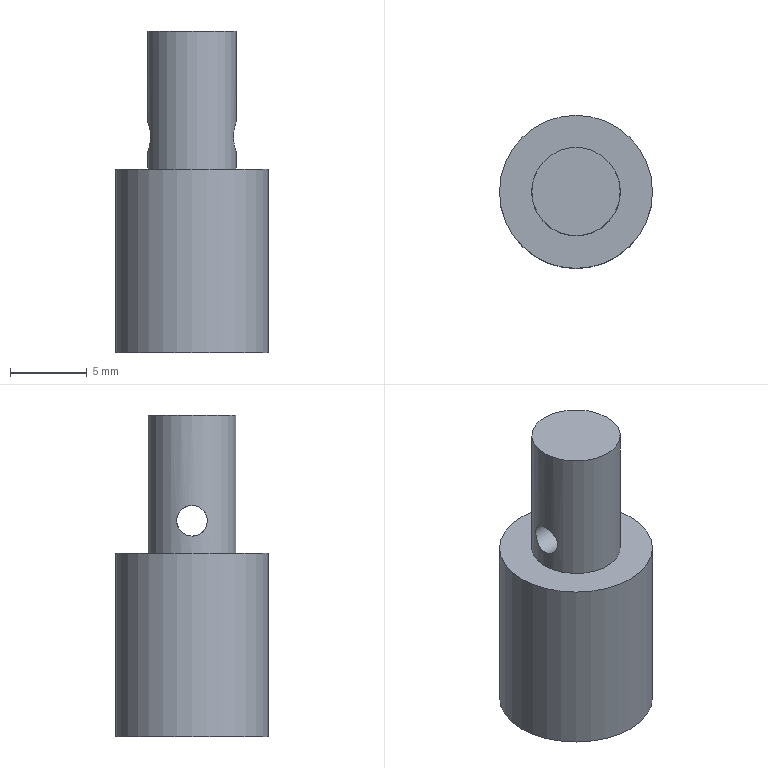Part | STEP file | Ground post | 1 solid | 6 faces | box 10 x 10 x 21 mm | volume 1161 mm3 | cylinder 3 | plane 3 | commonest cylinder face diameters 2 x1 5.78 x1 10 x1
STEP:
#1=CARTESIAN_POINT('',(0.,0.,0.));
#2=DIRECTION('',(0.,0.,1.));
#3=DIRECTION('',(1.,0.,0.));
#4=AXIS2_PLACEMENT_3D('',#1,#2,#3);
#5=CARTESIAN_POINT('',(2.89,0.,11.));
#6=VERTEX_POINT('',#5);
#7=CARTESIAN_POINT('',(0.,0.,11.));
#8=DIRECTION('',(0.,0.,1.));
#9=DIRECTION('',(1.,0.,0.));
#10=AXIS2_PLACEMENT_3D('',#7,#8,#9);
#11=CIRCLE('',#10,2.89);
#12=CARTESIAN_POINT('',(0.,0.,11.));
#13=DIRECTION('',(0.,0.,-1.));
#14=DIRECTION('',(-1.,0.,0.));
#15=AXIS2_PLACEMENT_3D('',#12,#13,#14);
#16=CYLINDRICAL_SURFACE('',#15,2.89);
#17=CARTESIAN_POINT('',(9.425,0.));
#18=DIRECTION('',(-1.,0.));
#19=VECTOR('',#18,1.);
#20=LINE('',#17,#19);
#21=(GEOMETRIC_REPRESENTATION_CONTEXT(2)PARAMETRIC_REPRESENTATION_CONTEXT()REPRESENTATION_CONTEXT('',''));
#22=DEFINITIONAL_REPRESENTATION('',(#20),#21);
#23=PCURVE('',#16,#22);
#24=CARTESIAN_POINT('',(0.,0.,11.));
#25=DIRECTION('',(0.,0.,1.));
#26=DIRECTION('',(1.,0.,0.));
#27=AXIS2_PLACEMENT_3D('',#24,#25,#26);
#28=PLANE('',#27);
#29=CARTESIAN_POINT('',(0.,0.));
#30=DIRECTION('',(1.,0.));
#31=AXIS2_PLACEMENT_2D('',#29,#30);
#32=CIRCLE('',#31,2.89);
#33=(GEOMETRIC_REPRESENTATION_CONTEXT(2)PARAMETRIC_REPRESENTATION_CONTEXT()REPRESENTATION_CONTEXT('',''));
#34=DEFINITIONAL_REPRESENTATION('',(#32),#33);
#35=PCURVE('',#28,#34);
#36=SURFACE_CURVE('',#11,(#23,#35),.PCURVE_S1.);
#37=EDGE_CURVE('',#6,#6,#36,.T.);
#38=ORIENTED_EDGE('',*,*,#37,.F.);
#39=CARTESIAN_POINT('',(2.89,0.,5.108));
#40=VERTEX_POINT('',#39);
#41=CARTESIAN_POINT('',(2.89,0.,11.));
#42=CARTESIAN_POINT('',(2.89,0.,5.108));
#43=B_SPLINE_CURVE_WITH_KNOTS('',1,(#41,#42),.UNSPECIFIED.,.F.,.F.,(2,2),(0.,5.892),.PIECEWISE_BEZIER_KNOTS.);
#44=CARTESIAN_POINT('',(9.425,0.));
#45=DIRECTION('',(0.,1.));
#46=VECTOR('',#45,1.);
#47=LINE('',#44,#46);
#48=(GEOMETRIC_REPRESENTATION_CONTEXT(2)PARAMETRIC_REPRESENTATION_CONTEXT()REPRESENTATION_CONTEXT('',''));
#49=DEFINITIONAL_REPRESENTATION('',(#47),#48);
#50=PCURVE('',#16,#49);
#51=CARTESIAN_POINT('',(3.142,0.));
#52=DIRECTION('',(0.,1.));
#53=VECTOR('',#52,1.);
#54=LINE('',#51,#53);
#55=(GEOMETRIC_REPRESENTATION_CONTEXT(2)PARAMETRIC_REPRESENTATION_CONTEXT()REPRESENTATION_CONTEXT('',''));
#56=DEFINITIONAL_REPRESENTATION('',(#54),#55);
#57=PCURVE('',#16,#56);
#58=SEAM_CURVE('',#43,(#50,#57),.PCURVE_S1.);
#59=EDGE_CURVE('',#6,#40,#58,.T.);
#60=ORIENTED_EDGE('',*,*,#59,.T.);
#61=CARTESIAN_POINT('',(2.89,0.,3.108));
#62=VERTEX_POINT('',#61);
#63=CARTESIAN_POINT('',(2.89,0.,5.108));
#64=CARTESIAN_POINT('',(2.89,-0.1084,5.108));
#65=CARTESIAN_POINT('',(2.884,-0.2182,5.09));
#66=CARTESIAN_POINT('',(2.872,-0.3203,5.055));
#67=CARTESIAN_POINT('',(2.861,-0.4222,5.021));
#68=CARTESIAN_POINT('',(2.844,-0.5192,4.969));
#69=CARTESIAN_POINT('',(2.826,-0.6042,4.904));
#70=CARTESIAN_POINT('',(2.807,-0.6921,4.838));
#71=CARTESIAN_POINT('',(2.786,-0.7695,4.756));
#72=CARTESIAN_POINT('',(2.768,-0.8309,4.664));
#73=CARTESIAN_POINT('',(2.749,-0.8942,4.57));
#74=CARTESIAN_POINT('',(2.732,-0.9421,4.462));
#75=CARTESIAN_POINT('',(2.722,-0.97,4.351));
#76=CARTESIAN_POINT('',(2.713,-0.9969,4.243));
#77=CARTESIAN_POINT('',(2.709,-1.006,4.129));
#78=CARTESIAN_POINT('',(2.713,-0.996,4.019));
#79=CARTESIAN_POINT('',(2.716,-0.9866,3.913));
#80=CARTESIAN_POINT('',(2.726,-0.96,3.809));
#81=CARTESIAN_POINT('',(2.74,-0.9186,3.712));
#82=CARTESIAN_POINT('',(2.754,-0.8765,3.615));
#83=CARTESIAN_POINT('',(2.773,-0.8181,3.523));
#84=CARTESIAN_POINT('',(2.792,-0.7479,3.444));
#85=CARTESIAN_POINT('',(2.811,-0.6737,3.36));
#86=CARTESIAN_POINT('',(2.832,-0.5842,3.288));
#87=CARTESIAN_POINT('',(2.849,-0.4861,3.234));
#88=CARTESIAN_POINT('',(2.866,-0.3869,3.179));
#89=CARTESIAN_POINT('',(2.879,-0.2759,3.14));
#90=CARTESIAN_POINT('',(2.885,-0.1628,3.121));
#91=CARTESIAN_POINT('',(2.891,-0.05501,3.103));
#92=CARTESIAN_POINT('',(2.891,0.05773,3.103));
#93=CARTESIAN_POINT('',(2.885,0.1655,3.121));
#94=CARTESIAN_POINT('',(2.879,0.2699,3.139));
#95=CARTESIAN_POINT('',(2.867,0.3724,3.174));
#96=CARTESIAN_POINT('',(2.852,0.4652,3.222));
#97=CARTESIAN_POINT('',(2.837,0.5607,3.273));
#98=CARTESIAN_POINT('',(2.817,0.6485,3.339));
#99=CARTESIAN_POINT('',(2.798,0.7227,3.416));
#100=CARTESIAN_POINT('',(2.778,0.8004,3.498));
#101=CARTESIAN_POINT('',(2.758,0.8653,3.594));
#102=CARTESIAN_POINT('',(2.742,0.9118,3.697));
#103=CARTESIAN_POINT('',(2.727,0.9582,3.8));
#104=CARTESIAN_POINT('',(2.716,0.9876,3.914));
#105=CARTESIAN_POINT('',(2.713,0.9968,4.027));
#106=CARTESIAN_POINT('',(2.709,1.005,4.135));
#107=CARTESIAN_POINT('',(2.713,0.9963,4.245));
#108=CARTESIAN_POINT('',(2.722,0.9703,4.35));
#109=CARTESIAN_POINT('',(2.731,0.9448,4.452));
#110=CARTESIAN_POINT('',(2.746,0.9027,4.55));
#111=CARTESIAN_POINT('',(2.763,0.8474,4.639));
#112=CARTESIAN_POINT('',(2.781,0.7896,4.731));
#113=CARTESIAN_POINT('',(2.801,0.7157,4.814));
#114=CARTESIAN_POINT('',(2.82,0.6314,4.883));
#115=CARTESIAN_POINT('',(2.84,0.5434,4.955));
#116=CARTESIAN_POINT('',(2.858,0.4413,5.012));
#117=CARTESIAN_POINT('',(2.871,0.3333,5.05));
#118=CARTESIAN_POINT('',(2.883,0.2275,5.088));
#119=CARTESIAN_POINT('',(2.89,0.1129,5.108));
#120=CARTESIAN_POINT('',(2.89,0.,5.108));
#121=B_SPLINE_CURVE_WITH_KNOTS('',3,(#63,#64,#65,#66,#67,#68,#69,#70,#71,#72,#73,#74,#75,#76,#77,#78,#79,#80,#81,#82,#83,#84,#85,#86,#87,#88,#89,#90,#91,#92,#93,#94,#95,#96,#97,#98,#99,#100,#101,#102,#103,#104,#105,#106,#107,#108,#109,#110,#111,#112,#113,#114,#115,#116,#117,#118,#119,#120),.UNSPECIFIED.,.T.,.F.,(1,3,3,3,3,3,3,3,3,3,3,3,3,3,3,3,3,3,3,3,3,1),(-0.0538,0.,0.05159,0.1031,0.1563,0.2112,0.2642,0.3144,0.3655,0.4195,0.4742,0.5263,0.5767,0.6285,0.6829,0.7374,0.7887,0.8388,0.8913,0.9462,1.,1.052),.UNSPECIFIED.);
#122=CARTESIAN_POINT('',(9.425,5.892));
#123=CARTESIAN_POINT('',(9.433,5.892));
#124=CARTESIAN_POINT('',(9.45,5.894));
#125=CARTESIAN_POINT('',(9.474,5.902));
#126=CARTESIAN_POINT('',(9.499,5.915));
#127=CARTESIAN_POINT('',(9.523,5.933));
#128=CARTESIAN_POINT('',(9.547,5.955));
#129=CARTESIAN_POINT('',(9.57,5.983));
#130=CARTESIAN_POINT('',(9.592,6.015));
#131=CARTESIAN_POINT('',(9.614,6.051));
#132=CARTESIAN_POINT('',(9.634,6.092));
#133=CARTESIAN_POINT('',(9.654,6.136));
#134=CARTESIAN_POINT('',(9.672,6.185));
#135=CARTESIAN_POINT('',(9.69,6.237));
#136=CARTESIAN_POINT('',(9.706,6.292));
#137=CARTESIAN_POINT('',(9.72,6.35));
#138=CARTESIAN_POINT('',(9.733,6.411));
#139=CARTESIAN_POINT('',(9.745,6.475));
#140=CARTESIAN_POINT('',(9.755,6.541));
#141=CARTESIAN_POINT('',(9.763,6.609));
#142=CARTESIAN_POINT('',(9.77,6.678));
#143=CARTESIAN_POINT('',(9.775,6.748));
#144=CARTESIAN_POINT('',(9.777,6.82));
#145=CARTESIAN_POINT('',(9.778,6.892));
#146=CARTESIAN_POINT('',(9.777,6.964));
#147=CARTESIAN_POINT('',(9.775,7.035));
#148=CARTESIAN_POINT('',(9.77,7.106));
#149=CARTESIAN_POINT('',(9.763,7.176));
#150=CARTESIAN_POINT('',(9.755,7.244));
#151=CARTESIAN_POINT('',(9.745,7.309));
#152=CARTESIAN_POINT('',(9.733,7.373));
#153=CARTESIAN_POINT('',(9.72,7.434));
#154=CARTESIAN_POINT('',(9.705,7.493));
#155=CARTESIAN_POINT('',(9.689,7.548));
#156=CARTESIAN_POINT('',(9.672,7.6));
#157=CARTESIAN_POINT('',(9.654,7.648));
#158=CARTESIAN_POINT('',(9.634,7.693));
#159=CARTESIAN_POINT('',(9.614,7.733));
#160=CARTESIAN_POINT('',(9.592,7.77));
#161=CARTESIAN_POINT('',(9.57,7.802));
#162=CARTESIAN_POINT('',(9.547,7.829));
#163=CARTESIAN_POINT('',(9.523,7.852));
#164=CARTESIAN_POINT('',(9.499,7.87));
#165=CARTESIAN_POINT('',(9.475,7.883));
#166=CARTESIAN_POINT('',(9.45,7.89));
#167=CARTESIAN_POINT('',(9.425,7.893));
#168=CARTESIAN_POINT('',(9.4,7.891));
#169=CARTESIAN_POINT('',(9.375,7.883));
#170=CARTESIAN_POINT('',(9.351,7.87));
#171=CARTESIAN_POINT('',(9.327,7.852));
#172=CARTESIAN_POINT('',(9.303,7.829));
#173=CARTESIAN_POINT('',(9.28,7.802));
#174=CARTESIAN_POINT('',(9.258,7.77));
#175=CARTESIAN_POINT('',(9.236,7.734));
#176=CARTESIAN_POINT('',(9.215,7.693));
#177=CARTESIAN_POINT('',(9.196,7.648));
#178=CARTESIAN_POINT('',(9.177,7.6));
#179=CARTESIAN_POINT('',(9.16,7.548));
#180=CARTESIAN_POINT('',(9.144,7.493));
#181=CARTESIAN_POINT('',(9.129,7.434));
#182=CARTESIAN_POINT('',(9.116,7.373));
#183=CARTESIAN_POINT('',(9.105,7.31));
#184=CARTESIAN_POINT('',(9.095,7.244));
#185=CARTESIAN_POINT('',(9.086,7.176));
#186=CARTESIAN_POINT('',(9.08,7.107));
#187=CARTESIAN_POINT('',(9.075,7.036));
#188=CARTESIAN_POINT('',(9.072,6.965));
#189=CARTESIAN_POINT('',(9.071,6.893));
#190=CARTESIAN_POINT('',(9.072,6.821));
#191=CARTESIAN_POINT('',(9.075,6.749));
#192=CARTESIAN_POINT('',(9.08,6.678));
#193=CARTESIAN_POINT('',(9.086,6.609));
#194=CARTESIAN_POINT('',(9.095,6.541));
#195=CARTESIAN_POINT('',(9.105,6.475));
#196=CARTESIAN_POINT('',(9.116,6.411));
#197=CARTESIAN_POINT('',(9.129,6.35));
#198=CARTESIAN_POINT('',(9.144,6.292));
#199=CARTESIAN_POINT('',(9.16,6.237));
#200=CARTESIAN_POINT('',(9.177,6.185));
#201=CARTESIAN_POINT('',(9.196,6.136));
#202=CARTESIAN_POINT('',(9.215,6.092));
#203=CARTESIAN_POINT('',(9.236,6.051));
#204=CARTESIAN_POINT('',(9.258,6.015));
#205=CARTESIAN_POINT('',(9.28,5.983));
#206=CARTESIAN_POINT('',(9.303,5.955));
#207=CARTESIAN_POINT('',(9.326,5.933));
#208=CARTESIAN_POINT('',(9.351,5.915));
#209=CARTESIAN_POINT('',(9.375,5.902));
#210=CARTESIAN_POINT('',(9.4,5.894));
#211=CARTESIAN_POINT('',(9.417,5.892));
#212=CARTESIAN_POINT('',(9.425,5.892));
#213=B_SPLINE_CURVE_WITH_KNOTS('',3,(#122,#123,#124,#125,#126,#127,#128,#129,#130,#131,#132,#133,#134,#135,#136,#137,#138,#139,#140,#141,#142,#143,#144,#145,#146,#147,#148,#149,#150,#151,#152,#153,#154,#155,#156,#157,#158,#159,#160,#161,#162,#163,#164,#165,#166,#167,#168,#169,#170,#171,#172,#173,#174,#175,#176,#177,#178,#179,#180,#181,#182,#183,#184,#185,#186,#187,#188,#189,#190,#191,#192,#193,#194,#195,#196,#197,#198,#199,#200,#201,#202,#203,#204,#205,#206,#207,#208,#209,#210,#211,#212),.UNSPECIFIED.,.T.,.F.,(4,1,1,1,1,1,1,1,1,1,1,1,1,1,1,1,1,1,1,1,1,1,1,1,1,1,1,1,1,1,1,1,1,1,1,1,1,1,1,1,1,1,1,1,1,1,1,1,1,1,1,1,1,1,1,1,1,1,1,1,1,1,1,1,1,1,1,1,1,1,1,1,1,1,1,1,1,1,1,1,1,1,1,1,1,1,1,1,4),(0.,0.01136,0.02273,0.03409,0.04545,0.05682,0.06818,0.07955,0.09091,0.1023,0.1136,0.125,0.1364,0.1477,0.1591,0.1705,0.1818,0.1932,0.2045,0.2159,0.2273,0.2386,0.25,0.2614,0.2727,0.2841,0.2955,0.3068,0.3182,0.3295,0.3409,0.3523,0.3636,0.375,0.3864,0.3977,0.4091,0.4205,0.4318,0.4432,0.4545,0.4659,0.4773,0.4886,0.5,0.5114,0.5227,0.5341,0.5455,0.5568,0.5682,0.5795,0.5909,0.6023,0.6136,0.625,0.6364,0.6477,0.6591,0.6705,0.6818,0.6932,0.7045,0.7159,0.7273,0.7386,0.75,0.7614,0.7727,0.7841,0.7955,0.8068,0.8182,0.8295,0.8409,0.8523,0.8636,0.875,0.8864,0.8977,0.9091,0.9205,0.9318,0.9432,0.9545,0.9659,0.9773,0.9886,1.),.QUASI_UNIFORM_KNOTS.);
#214=(GEOMETRIC_REPRESENTATION_CONTEXT(2)PARAMETRIC_REPRESENTATION_CONTEXT()REPRESENTATION_CONTEXT('',''));
#215=DEFINITIONAL_REPRESENTATION('',(#213),#214);
#216=PCURVE('',#16,#215);
#217=CARTESIAN_POINT('',(10.,0.,4.108));
#218=DIRECTION('',(-1.,0.,0.));
#219=DIRECTION('',(0.,0.,1.));
#220=AXIS2_PLACEMENT_3D('',#217,#218,#219);
#221=CYLINDRICAL_SURFACE('',#220,1.);
#222=CARTESIAN_POINT('',(3.142,7.11));
#223=CARTESIAN_POINT('',(3.118,7.11));
#224=CARTESIAN_POINT('',(3.069,7.111));
#225=CARTESIAN_POINT('',(2.998,7.113));
#226=CARTESIAN_POINT('',(2.926,7.118));
#227=CARTESIAN_POINT('',(2.854,7.124));
#228=CARTESIAN_POINT('',(2.782,7.131));
#229=CARTESIAN_POINT('',(2.711,7.14));
#230=CARTESIAN_POINT('',(2.64,7.15));
#231=CARTESIAN_POINT('',(2.569,7.161));
#232=CARTESIAN_POINT('',(2.498,7.173));
#233=CARTESIAN_POINT('',(2.426,7.185));
#234=CARTESIAN_POINT('',(2.356,7.198));
#235=CARTESIAN_POINT('',(2.285,7.211));
#236=CARTESIAN_POINT('',(2.214,7.223));
#237=CARTESIAN_POINT('',(2.143,7.235));
#238=CARTESIAN_POINT('',(2.072,7.246));
#239=CARTESIAN_POINT('',(2.001,7.257));
#240=CARTESIAN_POINT('',(1.93,7.266));
#241=CARTESIAN_POINT('',(1.858,7.274));
#242=CARTESIAN_POINT('',(1.786,7.28));
#243=CARTESIAN_POINT('',(1.714,7.285));
#244=CARTESIAN_POINT('',(1.643,7.288));
#245=CARTESIAN_POINT('',(1.571,7.289));
#246=CARTESIAN_POINT('',(1.499,7.288));
#247=CARTESIAN_POINT('',(1.427,7.285));
#248=CARTESIAN_POINT('',(1.355,7.28));
#249=CARTESIAN_POINT('',(1.284,7.274));
#250=CARTESIAN_POINT('',(1.212,7.266));
#251=CARTESIAN_POINT('',(1.14,7.257));
#252=CARTESIAN_POINT('',(1.069,7.246));
#253=CARTESIAN_POINT('',(0.9981,7.235));
#254=CARTESIAN_POINT('',(0.9272,7.223));
#255=CARTESIAN_POINT('',(0.8561,7.21));
#256=CARTESIAN_POINT('',(0.7851,7.198));
#257=CARTESIAN_POINT('',(0.7142,7.185));
#258=CARTESIAN_POINT('',(0.6436,7.173));
#259=CARTESIAN_POINT('',(0.5726,7.161));
#260=CARTESIAN_POINT('',(0.5013,7.15));
#261=CARTESIAN_POINT('',(0.43,7.14));
#262=CARTESIAN_POINT('',(0.3587,7.131));
#263=CARTESIAN_POINT('',(0.2875,7.124));
#264=CARTESIAN_POINT('',(0.2157,7.118));
#265=CARTESIAN_POINT('',(0.1437,7.113));
#266=CARTESIAN_POINT('',(0.07169,7.111));
#267=CARTESIAN_POINT('',(0.02384,7.11));
#268=CARTESIAN_POINT('',(0.,7.11));
#269=B_SPLINE_CURVE_WITH_KNOTS('',3,(#222,#223,#224,#225,#226,#227,#228,#229,#230,#231,#232,#233,#234,#235,#236,#237,#238,#239,#240,#241,#242,#243,#244,#245,#246,#247,#248,#249,#250,#251,#252,#253,#254,#255,#256,#257,#258,#259,#260,#261,#262,#263,#264,#265,#266,#267,#268),.UNSPECIFIED.,.F.,.F.,(4,1,1,1,1,1,1,1,1,1,1,1,1,1,1,1,1,1,1,1,1,1,1,1,1,1,1,1,1,1,1,1,1,1,1,1,1,1,1,1,1,1,1,1,4),(0.5001,0.5114,0.5228,0.5341,0.5455,0.5569,0.5682,0.5796,0.591,0.6023,0.6137,0.625,0.6364,0.6478,0.6591,0.6705,0.6819,0.6932,0.7046,0.7159,0.7273,0.7387,0.75,0.7614,0.7728,0.7841,0.7955,0.8068,0.8182,0.8296,0.8409,0.8523,0.8637,0.875,0.8864,0.8977,0.9091,0.9205,0.9318,0.9432,0.9546,0.9659,0.9773,0.9886,1.),.QUASI_UNIFORM_KNOTS.);
#270=(GEOMETRIC_REPRESENTATION_CONTEXT(2)PARAMETRIC_REPRESENTATION_CONTEXT()REPRESENTATION_CONTEXT('',''));
#271=DEFINITIONAL_REPRESENTATION('',(#269),#270);
#272=PCURVE('',#221,#271);
#273=SURFACE_CURVE('',#121,(#216,#272),.PCURVE_S1.);
#274=EDGE_CURVE('',#62,#40,#273,.T.);
#275=ORIENTED_EDGE('',*,*,#274,.F.);
#276=CARTESIAN_POINT('',(2.89,0.,2.));
#277=VERTEX_POINT('',#276);
#278=CARTESIAN_POINT('',(2.89,0.,3.108));
#279=CARTESIAN_POINT('',(2.89,0.,2.));
#280=B_SPLINE_CURVE_WITH_KNOTS('',1,(#278,#279),.UNSPECIFIED.,.F.,.F.,(2,2),(7.892,9.),.PIECEWISE_BEZIER_KNOTS.);
#281=CARTESIAN_POINT('',(9.425,0.));
#282=DIRECTION('',(0.,1.));
#283=VECTOR('',#282,1.);
#284=LINE('',#281,#283);
#285=(GEOMETRIC_REPRESENTATION_CONTEXT(2)PARAMETRIC_REPRESENTATION_CONTEXT()REPRESENTATION_CONTEXT('',''));
#286=DEFINITIONAL_REPRESENTATION('',(#284),#285);
#287=PCURVE('',#16,#286);
#288=CARTESIAN_POINT('',(3.142,0.));
#289=DIRECTION('',(0.,1.));
#290=VECTOR('',#289,1.);
#291=LINE('',#288,#290);
#292=(GEOMETRIC_REPRESENTATION_CONTEXT(2)PARAMETRIC_REPRESENTATION_CONTEXT()REPRESENTATION_CONTEXT('',''));
#293=DEFINITIONAL_REPRESENTATION('',(#291),#292);
#294=PCURVE('',#16,#293);
#295=SEAM_CURVE('',#280,(#287,#294),.PCURVE_S1.);
#296=EDGE_CURVE('',#62,#277,#295,.T.);
#297=ORIENTED_EDGE('',*,*,#296,.T.);
#298=CARTESIAN_POINT('',(0.,0.,2.));
#299=DIRECTION('',(0.,0.,1.));
#300=DIRECTION('',(1.,0.,0.));
#301=AXIS2_PLACEMENT_3D('',#298,#299,#300);
#302=CIRCLE('',#301,2.89);
#303=CARTESIAN_POINT('',(9.425,9.));
#304=DIRECTION('',(-1.,0.));
#305=VECTOR('',#304,1.);
#306=LINE('',#303,#305);
#307=(GEOMETRIC_REPRESENTATION_CONTEXT(2)PARAMETRIC_REPRESENTATION_CONTEXT()REPRESENTATION_CONTEXT('',''));
#308=DEFINITIONAL_REPRESENTATION('',(#306),#307);
#309=PCURVE('',#16,#308);
#310=CARTESIAN_POINT('',(0.,0.,2.));
#311=DIRECTION('',(0.,0.,1.));
#312=DIRECTION('',(1.,0.,0.));
#313=AXIS2_PLACEMENT_3D('',#310,#311,#312);
#314=PLANE('',#313);
#315=CARTESIAN_POINT('',(0.,0.));
#316=DIRECTION('',(1.,0.));
#317=AXIS2_PLACEMENT_2D('',#315,#316);
#318=CIRCLE('',#317,2.89);
#319=(GEOMETRIC_REPRESENTATION_CONTEXT(2)PARAMETRIC_REPRESENTATION_CONTEXT()REPRESENTATION_CONTEXT('',''));
#320=DEFINITIONAL_REPRESENTATION('',(#318),#319);
#321=PCURVE('',#314,#320);
#322=SURFACE_CURVE('',#302,(#309,#321),.PCURVE_S1.);
#323=EDGE_CURVE('',#277,#277,#322,.T.);
#324=ORIENTED_EDGE('',*,*,#323,.T.);
#325=ORIENTED_EDGE('',*,*,#296,.F.);
#326=CARTESIAN_POINT('',(2.89,0.,5.108));
#327=CARTESIAN_POINT('',(2.89,-0.1084,5.108));
#328=CARTESIAN_POINT('',(2.884,-0.2182,5.09));
#329=CARTESIAN_POINT('',(2.872,-0.3203,5.055));
#330=CARTESIAN_POINT('',(2.861,-0.4222,5.021));
#331=CARTESIAN_POINT('',(2.844,-0.5192,4.969));
#332=CARTESIAN_POINT('',(2.826,-0.6042,4.904));
#333=CARTESIAN_POINT('',(2.807,-0.6921,4.838));
#334=CARTESIAN_POINT('',(2.786,-0.7695,4.756));
#335=CARTESIAN_POINT('',(2.768,-0.8309,4.664));
#336=CARTESIAN_POINT('',(2.749,-0.8942,4.57));
#337=CARTESIAN_POINT('',(2.732,-0.9421,4.462));
#338=CARTESIAN_POINT('',(2.722,-0.97,4.351));
#339=CARTESIAN_POINT('',(2.713,-0.9969,4.243));
#340=CARTESIAN_POINT('',(2.709,-1.006,4.129));
#341=CARTESIAN_POINT('',(2.713,-0.996,4.019));
#342=CARTESIAN_POINT('',(2.716,-0.9866,3.913));
#343=CARTESIAN_POINT('',(2.726,-0.96,3.809));
#344=CARTESIAN_POINT('',(2.74,-0.9186,3.712));
#345=CARTESIAN_POINT('',(2.754,-0.8765,3.615));
#346=CARTESIAN_POINT('',(2.773,-0.8181,3.523));
#347=CARTESIAN_POINT('',(2.792,-0.7479,3.444));
#348=CARTESIAN_POINT('',(2.811,-0.6737,3.36));
#349=CARTESIAN_POINT('',(2.832,-0.5842,3.288));
#350=CARTESIAN_POINT('',(2.849,-0.4861,3.234));
#351=CARTESIAN_POINT('',(2.866,-0.3869,3.179));
#352=CARTESIAN_POINT('',(2.879,-0.2759,3.14));
#353=CARTESIAN_POINT('',(2.885,-0.1628,3.121));
#354=CARTESIAN_POINT('',(2.891,-0.05501,3.103));
#355=CARTESIAN_POINT('',(2.891,0.05773,3.103));
#356=CARTESIAN_POINT('',(2.885,0.1655,3.121));
#357=CARTESIAN_POINT('',(2.879,0.2699,3.139));
#358=CARTESIAN_POINT('',(2.867,0.3724,3.174));
#359=CARTESIAN_POINT('',(2.852,0.4652,3.222));
#360=CARTESIAN_POINT('',(2.837,0.5607,3.273));
#361=CARTESIAN_POINT('',(2.817,0.6485,3.339));
#362=CARTESIAN_POINT('',(2.798,0.7227,3.416));
#363=CARTESIAN_POINT('',(2.778,0.8004,3.498));
#364=CARTESIAN_POINT('',(2.758,0.8653,3.594));
#365=CARTESIAN_POINT('',(2.742,0.9118,3.697));
#366=CARTESIAN_POINT('',(2.727,0.9582,3.8));
#367=CARTESIAN_POINT('',(2.716,0.9876,3.914));
#368=CARTESIAN_POINT('',(2.713,0.9968,4.027));
#369=CARTESIAN_POINT('',(2.709,1.005,4.135));
#370=CARTESIAN_POINT('',(2.713,0.9963,4.245));
#371=CARTESIAN_POINT('',(2.722,0.9703,4.35));
#372=CARTESIAN_POINT('',(2.731,0.9448,4.452));
#373=CARTESIAN_POINT('',(2.746,0.9027,4.55));
#374=CARTESIAN_POINT('',(2.763,0.8474,4.639));
#375=CARTESIAN_POINT('',(2.781,0.7896,4.731));
#376=CARTESIAN_POINT('',(2.801,0.7157,4.814));
#377=CARTESIAN_POINT('',(2.82,0.6314,4.883));
#378=CARTESIAN_POINT('',(2.84,0.5434,4.955));
#379=CARTESIAN_POINT('',(2.858,0.4413,5.012));
#380=CARTESIAN_POINT('',(2.871,0.3333,5.05));
#381=CARTESIAN_POINT('',(2.883,0.2275,5.088));
#382=CARTESIAN_POINT('',(2.89,0.1129,5.108));
#383=CARTESIAN_POINT('',(2.89,0.,5.108));
#384=B_SPLINE_CURVE_WITH_KNOTS('',3,(#326,#327,#328,#329,#330,#331,#332,#333,#334,#335,#336,#337,#338,#339,#340,#341,#342,#343,#344,#345,#346,#347,#348,#349,#350,#351,#352,#353,#354,#355,#356,#357,#358,#359,#360,#361,#362,#363,#364,#365,#366,#367,#368,#369,#370,#371,#372,#373,#374,#375,#376,#377,#378,#379,#380,#381,#382,#383),.UNSPECIFIED.,.T.,.F.,(1,3,3,3,3,3,3,3,3,3,3,3,3,3,3,3,3,3,3,3,3,1),(-0.0538,0.,0.05159,0.1031,0.1563,0.2112,0.2642,0.3144,0.3655,0.4195,0.4742,0.5263,0.5767,0.6285,0.6829,0.7374,0.7887,0.8388,0.8913,0.9462,1.,1.052),.UNSPECIFIED.);
#385=CARTESIAN_POINT('',(3.142,5.892));
#386=CARTESIAN_POINT('',(3.15,5.892));
#387=CARTESIAN_POINT('',(3.166,5.894));
#388=CARTESIAN_POINT('',(3.191,5.902));
#389=CARTESIAN_POINT('',(3.216,5.915));
#390=CARTESIAN_POINT('',(3.24,5.933));
#391=CARTESIAN_POINT('',(3.263,5.955));
#392=CARTESIAN_POINT('',(3.287,5.983));
#393=CARTESIAN_POINT('',(3.309,6.015));
#394=CARTESIAN_POINT('',(3.33,6.051));
#395=CARTESIAN_POINT('',(3.351,6.092));
#396=CARTESIAN_POINT('',(3.371,6.136));
#397=CARTESIAN_POINT('',(3.389,6.185));
#398=CARTESIAN_POINT('',(3.406,6.237));
#399=CARTESIAN_POINT('',(3.422,6.292));
#400=CARTESIAN_POINT('',(3.437,6.35));
#401=CARTESIAN_POINT('',(3.45,6.411));
#402=CARTESIAN_POINT('',(3.462,6.475));
#403=CARTESIAN_POINT('',(3.472,6.541));
#404=CARTESIAN_POINT('',(3.48,6.609));
#405=CARTESIAN_POINT('',(3.487,6.678));
#406=CARTESIAN_POINT('',(3.491,6.748));
#407=CARTESIAN_POINT('',(3.494,6.82));
#408=CARTESIAN_POINT('',(3.495,6.892));
#409=CARTESIAN_POINT('',(3.494,6.964));
#410=CARTESIAN_POINT('',(3.491,7.035));
#411=CARTESIAN_POINT('',(3.487,7.106));
#412=CARTESIAN_POINT('',(3.48,7.176));
#413=CARTESIAN_POINT('',(3.472,7.244));
#414=CARTESIAN_POINT('',(3.462,7.309));
#415=CARTESIAN_POINT('',(3.45,7.373));
#416=CARTESIAN_POINT('',(3.437,7.434));
#417=CARTESIAN_POINT('',(3.422,7.493));
#418=CARTESIAN_POINT('',(3.406,7.548));
#419=CARTESIAN_POINT('',(3.389,7.6));
#420=CARTESIAN_POINT('',(3.371,7.648));
#421=CARTESIAN_POINT('',(3.351,7.693));
#422=CARTESIAN_POINT('',(3.33,7.733));
#423=CARTESIAN_POINT('',(3.309,7.77));
#424=CARTESIAN_POINT('',(3.287,7.802));
#425=CARTESIAN_POINT('',(3.264,7.829));
#426=CARTESIAN_POINT('',(3.24,7.852));
#427=CARTESIAN_POINT('',(3.216,7.87));
#428=CARTESIAN_POINT('',(3.191,7.883));
#429=CARTESIAN_POINT('',(3.167,7.89));
#430=CARTESIAN_POINT('',(3.142,7.893));
#431=CARTESIAN_POINT('',(3.117,7.891));
#432=CARTESIAN_POINT('',(3.092,7.883));
#433=CARTESIAN_POINT('',(3.068,7.87));
#434=CARTESIAN_POINT('',(3.043,7.852));
#435=CARTESIAN_POINT('',(3.02,7.829));
#436=CARTESIAN_POINT('',(2.997,7.802));
#437=CARTESIAN_POINT('',(2.974,7.77));
#438=CARTESIAN_POINT('',(2.953,7.734));
#439=CARTESIAN_POINT('',(2.932,7.693));
#440=CARTESIAN_POINT('',(2.913,7.648));
#441=CARTESIAN_POINT('',(2.894,7.6));
#442=CARTESIAN_POINT('',(2.877,7.548));
#443=CARTESIAN_POINT('',(2.861,7.493));
#444=CARTESIAN_POINT('',(2.846,7.434));
#445=CARTESIAN_POINT('',(2.833,7.373));
#446=CARTESIAN_POINT('',(2.821,7.31));
#447=CARTESIAN_POINT('',(2.811,7.244));
#448=CARTESIAN_POINT('',(2.803,7.176));
#449=CARTESIAN_POINT('',(2.797,7.107));
#450=CARTESIAN_POINT('',(2.792,7.036));
#451=CARTESIAN_POINT('',(2.789,6.965));
#452=CARTESIAN_POINT('',(2.788,6.893));
#453=CARTESIAN_POINT('',(2.789,6.821));
#454=CARTESIAN_POINT('',(2.792,6.749));
#455=CARTESIAN_POINT('',(2.796,6.678));
#456=CARTESIAN_POINT('',(2.803,6.609));
#457=CARTESIAN_POINT('',(2.811,6.541));
#458=CARTESIAN_POINT('',(2.821,6.475));
#459=CARTESIAN_POINT('',(2.833,6.411));
#460=CARTESIAN_POINT('',(2.846,6.35));
#461=CARTESIAN_POINT('',(2.861,6.292));
#462=CARTESIAN_POINT('',(2.877,6.237));
#463=CARTESIAN_POINT('',(2.894,6.185));
#464=CARTESIAN_POINT('',(2.913,6.136));
#465=CARTESIAN_POINT('',(2.932,6.092));
#466=CARTESIAN_POINT('',(2.953,6.051));
#467=CARTESIAN_POINT('',(2.974,6.015));
#468=CARTESIAN_POINT('',(2.997,5.983));
#469=CARTESIAN_POINT('',(3.02,5.955));
#470=CARTESIAN_POINT('',(3.043,5.933));
#471=CARTESIAN_POINT('',(3.067,5.915));
#472=CARTESIAN_POINT('',(3.092,5.902));
#473=CARTESIAN_POINT('',(3.117,5.894));
#474=CARTESIAN_POINT('',(3.133,5.892));
#475=CARTESIAN_POINT('',(3.142,5.892));
#476=B_SPLINE_CURVE_WITH_KNOTS('',3,(#385,#386,#387,#388,#389,#390,#391,#392,#393,#394,#395,#396,#397,#398,#399,#400,#401,#402,#403,#404,#405,#406,#407,#408,#409,#410,#411,#412,#413,#414,#415,#416,#417,#418,#419,#420,#421,#422,#423,#424,#425,#426,#427,#428,#429,#430,#431,#432,#433,#434,#435,#436,#437,#438,#439,#440,#441,#442,#443,#444,#445,#446,#447,#448,#449,#450,#451,#452,#453,#454,#455,#456,#457,#458,#459,#460,#461,#462,#463,#464,#465,#466,#467,#468,#469,#470,#471,#472,#473,#474,#475),.UNSPECIFIED.,.T.,.F.,(4,1,1,1,1,1,1,1,1,1,1,1,1,1,1,1,1,1,1,1,1,1,1,1,1,1,1,1,1,1,1,1,1,1,1,1,1,1,1,1,1,1,1,1,1,1,1,1,1,1,1,1,1,1,1,1,1,1,1,1,1,1,1,1,1,1,1,1,1,1,1,1,1,1,1,1,1,1,1,1,1,1,1,1,1,1,1,1,4),(0.,0.01136,0.02273,0.03409,0.04545,0.05682,0.06818,0.07955,0.09091,0.1023,0.1136,0.125,0.1364,0.1477,0.1591,0.1705,0.1818,0.1932,0.2045,0.2159,0.2273,0.2386,0.25,0.2614,0.2727,0.2841,0.2955,0.3068,0.3182,0.3295,0.3409,0.3523,0.3636,0.375,0.3864,0.3977,0.4091,0.4205,0.4318,0.4432,0.4545,0.4659,0.4773,0.4886,0.5,0.5114,0.5227,0.5341,0.5455,0.5568,0.5682,0.5795,0.5909,0.6023,0.6136,0.625,0.6364,0.6477,0.6591,0.6705,0.6818,0.6932,0.7045,0.7159,0.7273,0.7386,0.75,0.7614,0.7727,0.7841,0.7955,0.8068,0.8182,0.8295,0.8409,0.8523,0.8636,0.875,0.8864,0.8977,0.9091,0.9205,0.9318,0.9432,0.9545,0.9659,0.9773,0.9886,1.),.QUASI_UNIFORM_KNOTS.);
#477=(GEOMETRIC_REPRESENTATION_CONTEXT(2)PARAMETRIC_REPRESENTATION_CONTEXT()REPRESENTATION_CONTEXT('',''));
#478=DEFINITIONAL_REPRESENTATION('',(#476),#477);
#479=PCURVE('',#16,#478);
#480=CARTESIAN_POINT('',(6.283,7.11));
#481=CARTESIAN_POINT('',(6.259,7.11));
#482=CARTESIAN_POINT('',(6.211,7.111));
#483=CARTESIAN_POINT('',(6.139,7.113));
#484=CARTESIAN_POINT('',(6.067,7.118));
#485=CARTESIAN_POINT('',(5.996,7.124));
#486=CARTESIAN_POINT('',(5.924,7.131));
#487=CARTESIAN_POINT('',(5.853,7.14));
#488=CARTESIAN_POINT('',(5.781,7.15));
#489=CARTESIAN_POINT('',(5.71,7.161));
#490=CARTESIAN_POINT('',(5.639,7.173));
#491=CARTESIAN_POINT('',(5.569,7.185));
#492=CARTESIAN_POINT('',(5.497,7.198));
#493=CARTESIAN_POINT('',(5.426,7.211));
#494=CARTESIAN_POINT('',(5.355,7.223));
#495=CARTESIAN_POINT('',(5.285,7.235));
#496=CARTESIAN_POINT('',(5.214,7.246));
#497=CARTESIAN_POINT('',(5.143,7.257));
#498=CARTESIAN_POINT('',(5.071,7.266));
#499=CARTESIAN_POINT('',(5.,7.274));
#500=CARTESIAN_POINT('',(4.928,7.28));
#501=CARTESIAN_POINT('',(4.857,7.285));
#502=CARTESIAN_POINT('',(4.784,7.288));
#503=CARTESIAN_POINT('',(4.712,7.289));
#504=CARTESIAN_POINT('',(4.641,7.288));
#505=CARTESIAN_POINT('',(4.569,7.285));
#506=CARTESIAN_POINT('',(4.497,7.28));
#507=CARTESIAN_POINT('',(4.425,7.274));
#508=CARTESIAN_POINT('',(4.353,7.266));
#509=CARTESIAN_POINT('',(4.282,7.257));
#510=CARTESIAN_POINT('',(4.211,7.246));
#511=CARTESIAN_POINT('',(4.14,7.235));
#512=CARTESIAN_POINT('',(4.069,7.223));
#513=CARTESIAN_POINT('',(3.998,7.21));
#514=CARTESIAN_POINT('',(3.927,7.198));
#515=CARTESIAN_POINT('',(3.856,7.185));
#516=CARTESIAN_POINT('',(3.785,7.173));
#517=CARTESIAN_POINT('',(3.714,7.161));
#518=CARTESIAN_POINT('',(3.643,7.15));
#519=CARTESIAN_POINT('',(3.572,7.14));
#520=CARTESIAN_POINT('',(3.5,7.131));
#521=CARTESIAN_POINT('',(3.429,7.124));
#522=CARTESIAN_POINT('',(3.357,7.118));
#523=CARTESIAN_POINT('',(3.286,7.113));
#524=CARTESIAN_POINT('',(3.214,7.111));
#525=CARTESIAN_POINT('',(3.166,7.11));
#526=CARTESIAN_POINT('',(3.142,7.11));
#527=B_SPLINE_CURVE_WITH_KNOTS('',3,(#480,#481,#482,#483,#484,#485,#486,#487,#488,#489,#490,#491,#492,#493,#494,#495,#496,#497,#498,#499,#500,#501,#502,#503,#504,#505,#506,#507,#508,#509,#510,#511,#512,#513,#514,#515,#516,#517,#518,#519,#520,#521,#522,#523,#524,#525,#526),.UNSPECIFIED.,.F.,.F.,(4,1,1,1,1,1,1,1,1,1,1,1,1,1,1,1,1,1,1,1,1,1,1,1,1,1,1,1,1,1,1,1,1,1,1,1,1,1,1,1,1,1,1,1,4),(0.,0.01137,0.02273,0.0341,0.04546,0.05683,0.06819,0.07956,0.09092,0.1023,0.1137,0.125,0.1364,0.1477,0.1591,0.1705,0.1818,0.1932,0.2046,0.2159,0.2273,0.2387,0.25,0.2614,0.2728,0.2841,0.2955,0.3069,0.3182,0.3296,0.341,0.3523,0.3637,0.375,0.3864,0.3978,0.4091,0.4205,0.4319,0.4432,0.4546,0.466,0.4773,0.4887,0.5001),.QUASI_UNIFORM_KNOTS.);
#528=(GEOMETRIC_REPRESENTATION_CONTEXT(2)PARAMETRIC_REPRESENTATION_CONTEXT()REPRESENTATION_CONTEXT('',''));
#529=DEFINITIONAL_REPRESENTATION('',(#527),#528);
#530=PCURVE('',#221,#529);
#531=SURFACE_CURVE('',#384,(#479,#530),.PCURVE_S1.);
#532=EDGE_CURVE('',#40,#62,#531,.T.);
#533=ORIENTED_EDGE('',*,*,#532,.F.);
#534=ORIENTED_EDGE('',*,*,#59,.F.);
#535=EDGE_LOOP('',(#38,#60,#275,#297,#324,#325,#533,#534));
#536=FACE_BOUND('',#535,.T.);
#537=CARTESIAN_POINT('',(-2.89,0.,5.108));
#538=VERTEX_POINT('',#537);
#539=CARTESIAN_POINT('',(-2.89,0.,5.108));
#540=CARTESIAN_POINT('',(-2.89,0.1084,5.108));
#541=CARTESIAN_POINT('',(-2.884,0.2182,5.09));
#542=CARTESIAN_POINT('',(-2.872,0.3203,5.055));
#543=CARTESIAN_POINT('',(-2.861,0.4222,5.021));
#544=CARTESIAN_POINT('',(-2.844,0.5192,4.969));
#545=CARTESIAN_POINT('',(-2.826,0.6042,4.904));
#546=CARTESIAN_POINT('',(-2.807,0.6921,4.838));
#547=CARTESIAN_POINT('',(-2.786,0.7695,4.756));
#548=CARTESIAN_POINT('',(-2.768,0.8309,4.664));
#549=CARTESIAN_POINT('',(-2.749,0.8942,4.57));
#550=CARTESIAN_POINT('',(-2.732,0.9421,4.462));
#551=CARTESIAN_POINT('',(-2.722,0.97,4.351));
#552=CARTESIAN_POINT('',(-2.713,0.9969,4.243));
#553=CARTESIAN_POINT('',(-2.709,1.006,4.129));
#554=CARTESIAN_POINT('',(-2.713,0.996,4.019));
#555=CARTESIAN_POINT('',(-2.716,0.9866,3.913));
#556=CARTESIAN_POINT('',(-2.726,0.96,3.809));
#557=CARTESIAN_POINT('',(-2.74,0.9186,3.712));
#558=CARTESIAN_POINT('',(-2.754,0.8765,3.615));
#559=CARTESIAN_POINT('',(-2.773,0.8181,3.523));
#560=CARTESIAN_POINT('',(-2.792,0.7479,3.444));
#561=CARTESIAN_POINT('',(-2.811,0.6737,3.36));
#562=CARTESIAN_POINT('',(-2.832,0.5842,3.288));
#563=CARTESIAN_POINT('',(-2.849,0.4861,3.234));
#564=CARTESIAN_POINT('',(-2.866,0.3869,3.179));
#565=CARTESIAN_POINT('',(-2.879,0.2759,3.14));
#566=CARTESIAN_POINT('',(-2.885,0.1628,3.121));
#567=CARTESIAN_POINT('',(-2.891,0.05501,3.103));
#568=CARTESIAN_POINT('',(-2.891,-0.05773,3.103));
#569=CARTESIAN_POINT('',(-2.885,-0.1655,3.121));
#570=CARTESIAN_POINT('',(-2.879,-0.2699,3.139));
#571=CARTESIAN_POINT('',(-2.867,-0.3724,3.174));
#572=CARTESIAN_POINT('',(-2.852,-0.4652,3.222));
#573=CARTESIAN_POINT('',(-2.837,-0.5607,3.273));
#574=CARTESIAN_POINT('',(-2.817,-0.6485,3.339));
#575=CARTESIAN_POINT('',(-2.798,-0.7227,3.416));
#576=CARTESIAN_POINT('',(-2.778,-0.8004,3.498));
#577=CARTESIAN_POINT('',(-2.758,-0.8653,3.594));
#578=CARTESIAN_POINT('',(-2.742,-0.9118,3.697));
#579=CARTESIAN_POINT('',(-2.727,-0.9582,3.8));
#580=CARTESIAN_POINT('',(-2.716,-0.9876,3.914));
#581=CARTESIAN_POINT('',(-2.713,-0.9968,4.027));
#582=CARTESIAN_POINT('',(-2.709,-1.005,4.135));
#583=CARTESIAN_POINT('',(-2.713,-0.9963,4.245));
#584=CARTESIAN_POINT('',(-2.722,-0.9703,4.35));
#585=CARTESIAN_POINT('',(-2.731,-0.9448,4.452));
#586=CARTESIAN_POINT('',(-2.746,-0.9027,4.55));
#587=CARTESIAN_POINT('',(-2.763,-0.8474,4.639));
#588=CARTESIAN_POINT('',(-2.781,-0.7896,4.731));
#589=CARTESIAN_POINT('',(-2.801,-0.7157,4.814));
#590=CARTESIAN_POINT('',(-2.82,-0.6314,4.883));
#591=CARTESIAN_POINT('',(-2.84,-0.5434,4.955));
#592=CARTESIAN_POINT('',(-2.858,-0.4413,5.012));
#593=CARTESIAN_POINT('',(-2.871,-0.3333,5.05));
#594=CARTESIAN_POINT('',(-2.883,-0.2275,5.088));
#595=CARTESIAN_POINT('',(-2.89,-0.1129,5.108));
#596=CARTESIAN_POINT('',(-2.89,0.,5.108));
#597=B_SPLINE_CURVE_WITH_KNOTS('',3,(#539,#540,#541,#542,#543,#544,#545,#546,#547,#548,#549,#550,#551,#552,#553,#554,#555,#556,#557,#558,#559,#560,#561,#562,#563,#564,#565,#566,#567,#568,#569,#570,#571,#572,#573,#574,#575,#576,#577,#578,#579,#580,#581,#582,#583,#584,#585,#586,#587,#588,#589,#590,#591,#592,#593,#594,#595,#596),.UNSPECIFIED.,.T.,.F.,(1,3,3,3,3,3,3,3,3,3,3,3,3,3,3,3,3,3,3,3,3,1),(-0.0538,0.,0.05159,0.1031,0.1563,0.2112,0.2642,0.3144,0.3655,0.4195,0.4742,0.5263,0.5767,0.6285,0.6829,0.7374,0.7887,0.8388,0.8913,0.9462,1.,1.052),.UNSPECIFIED.);
#598=CARTESIAN_POINT('',(6.283,5.892));
#599=CARTESIAN_POINT('',(6.291,5.892));
#600=CARTESIAN_POINT('',(6.308,5.894));
#601=CARTESIAN_POINT('',(6.333,5.902));
#602=CARTESIAN_POINT('',(6.357,5.915));
#603=CARTESIAN_POINT('',(6.382,5.933));
#604=CARTESIAN_POINT('',(6.405,5.955));
#605=CARTESIAN_POINT('',(6.428,5.983));
#606=CARTESIAN_POINT('',(6.45,6.015));
#607=CARTESIAN_POINT('',(6.472,6.051));
#608=CARTESIAN_POINT('',(6.493,6.092));
#609=CARTESIAN_POINT('',(6.512,6.136));
#610=CARTESIAN_POINT('',(6.531,6.185));
#611=CARTESIAN_POINT('',(6.548,6.237));
#612=CARTESIAN_POINT('',(6.564,6.292));
#613=CARTESIAN_POINT('',(6.579,6.35));
#614=CARTESIAN_POINT('',(6.592,6.411));
#615=CARTESIAN_POINT('',(6.603,6.475));
#616=CARTESIAN_POINT('',(6.613,6.541));
#617=CARTESIAN_POINT('',(6.622,6.609));
#618=CARTESIAN_POINT('',(6.628,6.678));
#619=CARTESIAN_POINT('',(6.633,6.748));
#620=CARTESIAN_POINT('',(6.636,6.82));
#621=CARTESIAN_POINT('',(6.637,6.892));
#622=CARTESIAN_POINT('',(6.636,6.964));
#623=CARTESIAN_POINT('',(6.633,7.035));
#624=CARTESIAN_POINT('',(6.628,7.106));
#625=CARTESIAN_POINT('',(6.622,7.176));
#626=CARTESIAN_POINT('',(6.613,7.244));
#627=CARTESIAN_POINT('',(6.603,7.309));
#628=CARTESIAN_POINT('',(6.592,7.373));
#629=CARTESIAN_POINT('',(6.579,7.434));
#630=CARTESIAN_POINT('',(6.564,7.493));
#631=CARTESIAN_POINT('',(6.548,7.548));
#632=CARTESIAN_POINT('',(6.531,7.6));
#633=CARTESIAN_POINT('',(6.512,7.648));
#634=CARTESIAN_POINT('',(6.493,7.693));
#635=CARTESIAN_POINT('',(6.472,7.733));
#636=CARTESIAN_POINT('',(6.451,7.77));
#637=CARTESIAN_POINT('',(6.428,7.802));
#638=CARTESIAN_POINT('',(6.405,7.829));
#639=CARTESIAN_POINT('',(6.382,7.852));
#640=CARTESIAN_POINT('',(6.357,7.87));
#641=CARTESIAN_POINT('',(6.333,7.883));
#642=CARTESIAN_POINT('',(6.308,7.89));
#643=CARTESIAN_POINT('',(6.283,7.893));
#644=CARTESIAN_POINT('',(6.258,7.891));
#645=CARTESIAN_POINT('',(6.234,7.883));
#646=CARTESIAN_POINT('',(6.209,7.87));
#647=CARTESIAN_POINT('',(6.185,7.852));
#648=CARTESIAN_POINT('',(6.161,7.829));
#649=CARTESIAN_POINT('',(6.138,7.802));
#650=CARTESIAN_POINT('',(6.116,7.77));
#651=CARTESIAN_POINT('',(6.094,7.734));
#652=CARTESIAN_POINT('',(6.074,7.693));
#653=CARTESIAN_POINT('',(6.054,7.648));
#654=CARTESIAN_POINT('',(6.036,7.6));
#655=CARTESIAN_POINT('',(6.019,7.548));
#656=CARTESIAN_POINT('',(6.003,7.493));
#657=CARTESIAN_POINT('',(5.988,7.434));
#658=CARTESIAN_POINT('',(5.975,7.373));
#659=CARTESIAN_POINT('',(5.963,7.31));
#660=CARTESIAN_POINT('',(5.953,7.244));
#661=CARTESIAN_POINT('',(5.945,7.176));
#662=CARTESIAN_POINT('',(5.938,7.107));
#663=CARTESIAN_POINT('',(5.933,7.036));
#664=CARTESIAN_POINT('',(5.93,6.965));
#665=CARTESIAN_POINT('',(5.93,6.893));
#666=CARTESIAN_POINT('',(5.931,6.821));
#667=CARTESIAN_POINT('',(5.933,6.749));
#668=CARTESIAN_POINT('',(5.938,6.678));
#669=CARTESIAN_POINT('',(5.945,6.609));
#670=CARTESIAN_POINT('',(5.953,6.541));
#671=CARTESIAN_POINT('',(5.963,6.475));
#672=CARTESIAN_POINT('',(5.975,6.411));
#673=CARTESIAN_POINT('',(5.988,6.35));
#674=CARTESIAN_POINT('',(6.002,6.292));
#675=CARTESIAN_POINT('',(6.019,6.237));
#676=CARTESIAN_POINT('',(6.036,6.185));
#677=CARTESIAN_POINT('',(6.054,6.136));
#678=CARTESIAN_POINT('',(6.074,6.092));
#679=CARTESIAN_POINT('',(6.094,6.051));
#680=CARTESIAN_POINT('',(6.116,6.015));
#681=CARTESIAN_POINT('',(6.138,5.983));
#682=CARTESIAN_POINT('',(6.161,5.955));
#683=CARTESIAN_POINT('',(6.185,5.933));
#684=CARTESIAN_POINT('',(6.209,5.915));
#685=CARTESIAN_POINT('',(6.234,5.902));
#686=CARTESIAN_POINT('',(6.258,5.894));
#687=CARTESIAN_POINT('',(6.275,5.892));
#688=CARTESIAN_POINT('',(6.283,5.892));
#689=B_SPLINE_CURVE_WITH_KNOTS('',3,(#598,#599,#600,#601,#602,#603,#604,#605,#606,#607,#608,#609,#610,#611,#612,#613,#614,#615,#616,#617,#618,#619,#620,#621,#622,#623,#624,#625,#626,#627,#628,#629,#630,#631,#632,#633,#634,#635,#636,#637,#638,#639,#640,#641,#642,#643,#644,#645,#646,#647,#648,#649,#650,#651,#652,#653,#654,#655,#656,#657,#658,#659,#660,#661,#662,#663,#664,#665,#666,#667,#668,#669,#670,#671,#672,#673,#674,#675,#676,#677,#678,#679,#680,#681,#682,#683,#684,#685,#686,#687,#688),.UNSPECIFIED.,.T.,.F.,(4,1,1,1,1,1,1,1,1,1,1,1,1,1,1,1,1,1,1,1,1,1,1,1,1,1,1,1,1,1,1,1,1,1,1,1,1,1,1,1,1,1,1,1,1,1,1,1,1,1,1,1,1,1,1,1,1,1,1,1,1,1,1,1,1,1,1,1,1,1,1,1,1,1,1,1,1,1,1,1,1,1,1,1,1,1,1,1,4),(0.,0.01136,0.02273,0.03409,0.04545,0.05682,0.06818,0.07955,0.09091,0.1023,0.1136,0.125,0.1364,0.1477,0.1591,0.1705,0.1818,0.1932,0.2045,0.2159,0.2273,0.2386,0.25,0.2614,0.2727,0.2841,0.2955,0.3068,0.3182,0.3295,0.3409,0.3523,0.3636,0.375,0.3864,0.3977,0.4091,0.4205,0.4318,0.4432,0.4545,0.4659,0.4773,0.4886,0.5,0.5114,0.5227,0.5341,0.5455,0.5568,0.5682,0.5795,0.5909,0.6023,0.6136,0.625,0.6364,0.6477,0.6591,0.6705,0.6818,0.6932,0.7045,0.7159,0.7273,0.7386,0.75,0.7614,0.7727,0.7841,0.7955,0.8068,0.8182,0.8295,0.8409,0.8523,0.8636,0.875,0.8864,0.8977,0.9091,0.9205,0.9318,0.9432,0.9545,0.9659,0.9773,0.9886,1.),.QUASI_UNIFORM_KNOTS.);
#690=(GEOMETRIC_REPRESENTATION_CONTEXT(2)PARAMETRIC_REPRESENTATION_CONTEXT()REPRESENTATION_CONTEXT('',''));
#691=DEFINITIONAL_REPRESENTATION('',(#689),#690);
#692=PCURVE('',#16,#691);
#693=CARTESIAN_POINT('',(0.,12.89));
#694=CARTESIAN_POINT('',(0.02387,12.89));
#695=CARTESIAN_POINT('',(0.07175,12.889));
#696=CARTESIAN_POINT('',(0.1438,12.887));
#697=CARTESIAN_POINT('',(0.2158,12.882));
#698=CARTESIAN_POINT('',(0.2876,12.876));
#699=CARTESIAN_POINT('',(0.3588,12.869));
#700=CARTESIAN_POINT('',(0.4303,12.86));
#701=CARTESIAN_POINT('',(0.5017,12.85));
#702=CARTESIAN_POINT('',(0.573,12.839));
#703=CARTESIAN_POINT('',(0.6439,12.827));
#704=CARTESIAN_POINT('',(0.7146,12.815));
#705=CARTESIAN_POINT('',(0.7856,12.802));
#706=CARTESIAN_POINT('',(0.8566,12.789));
#707=CARTESIAN_POINT('',(0.9276,12.777));
#708=CARTESIAN_POINT('',(0.9982,12.765));
#709=CARTESIAN_POINT('',(1.069,12.754));
#710=CARTESIAN_POINT('',(1.14,12.743));
#711=CARTESIAN_POINT('',(1.212,12.734));
#712=CARTESIAN_POINT('',(1.283,12.726));
#713=CARTESIAN_POINT('',(1.355,12.72));
#714=CARTESIAN_POINT('',(1.426,12.715));
#715=CARTESIAN_POINT('',(1.499,12.712));
#716=CARTESIAN_POINT('',(1.571,12.711));
#717=CARTESIAN_POINT('',(1.642,12.712));
#718=CARTESIAN_POINT('',(1.714,12.715));
#719=CARTESIAN_POINT('',(1.786,12.72));
#720=CARTESIAN_POINT('',(1.858,12.726));
#721=CARTESIAN_POINT('',(1.93,12.734));
#722=CARTESIAN_POINT('',(2.001,12.743));
#723=CARTESIAN_POINT('',(2.072,12.754));
#724=CARTESIAN_POINT('',(2.143,12.765));
#725=CARTESIAN_POINT('',(2.214,12.777));
#726=CARTESIAN_POINT('',(2.285,12.789));
#727=CARTESIAN_POINT('',(2.356,12.802));
#728=CARTESIAN_POINT('',(2.427,12.815));
#729=CARTESIAN_POINT('',(2.498,12.827));
#730=CARTESIAN_POINT('',(2.569,12.839));
#731=CARTESIAN_POINT('',(2.64,12.85));
#732=CARTESIAN_POINT('',(2.711,12.86));
#733=CARTESIAN_POINT('',(2.782,12.869));
#734=CARTESIAN_POINT('',(2.854,12.876));
#735=CARTESIAN_POINT('',(2.926,12.882));
#736=CARTESIAN_POINT('',(2.997,12.887));
#737=CARTESIAN_POINT('',(3.069,12.889));
#738=CARTESIAN_POINT('',(3.141,12.89));
#739=CARTESIAN_POINT('',(3.213,12.889));
#740=CARTESIAN_POINT('',(3.285,12.887));
#741=CARTESIAN_POINT('',(3.357,12.882));
#742=CARTESIAN_POINT('',(3.429,12.876));
#743=CARTESIAN_POINT('',(3.5,12.869));
#744=CARTESIAN_POINT('',(3.572,12.86));
#745=CARTESIAN_POINT('',(3.643,12.85));
#746=CARTESIAN_POINT('',(3.714,12.839));
#747=CARTESIAN_POINT('',(3.785,12.827));
#748=CARTESIAN_POINT('',(3.856,12.815));
#749=CARTESIAN_POINT('',(3.927,12.802));
#750=CARTESIAN_POINT('',(3.998,12.79));
#751=CARTESIAN_POINT('',(4.069,12.777));
#752=CARTESIAN_POINT('',(4.14,12.765));
#753=CARTESIAN_POINT('',(4.211,12.754));
#754=CARTESIAN_POINT('',(4.282,12.743));
#755=CARTESIAN_POINT('',(4.353,12.734));
#756=CARTESIAN_POINT('',(4.425,12.726));
#757=CARTESIAN_POINT('',(4.497,12.72));
#758=CARTESIAN_POINT('',(4.569,12.715));
#759=CARTESIAN_POINT('',(4.64,12.712));
#760=CARTESIAN_POINT('',(4.712,12.711));
#761=CARTESIAN_POINT('',(4.784,12.712));
#762=CARTESIAN_POINT('',(4.856,12.715));
#763=CARTESIAN_POINT('',(4.928,12.72));
#764=CARTESIAN_POINT('',(4.999,12.726));
#765=CARTESIAN_POINT('',(5.071,12.734));
#766=CARTESIAN_POINT('',(5.143,12.743));
#767=CARTESIAN_POINT('',(5.214,12.754));
#768=CARTESIAN_POINT('',(5.285,12.765));
#769=CARTESIAN_POINT('',(5.356,12.777));
#770=CARTESIAN_POINT('',(5.427,12.79));
#771=CARTESIAN_POINT('',(5.498,12.802));
#772=CARTESIAN_POINT('',(5.569,12.815));
#773=CARTESIAN_POINT('',(5.639,12.827));
#774=CARTESIAN_POINT('',(5.71,12.839));
#775=CARTESIAN_POINT('',(5.782,12.85));
#776=CARTESIAN_POINT('',(5.853,12.86));
#777=CARTESIAN_POINT('',(5.924,12.869));
#778=CARTESIAN_POINT('',(5.996,12.876));
#779=CARTESIAN_POINT('',(6.067,12.882));
#780=CARTESIAN_POINT('',(6.139,12.887));
#781=CARTESIAN_POINT('',(6.211,12.889));
#782=CARTESIAN_POINT('',(6.259,12.89));
#783=CARTESIAN_POINT('',(6.283,12.89));
#784=B_SPLINE_CURVE_WITH_KNOTS('',3,(#693,#694,#695,#696,#697,#698,#699,#700,#701,#702,#703,#704,#705,#706,#707,#708,#709,#710,#711,#712,#713,#714,#715,#716,#717,#718,#719,#720,#721,#722,#723,#724,#725,#726,#727,#728,#729,#730,#731,#732,#733,#734,#735,#736,#737,#738,#739,#740,#741,#742,#743,#744,#745,#746,#747,#748,#749,#750,#751,#752,#753,#754,#755,#756,#757,#758,#759,#760,#761,#762,#763,#764,#765,#766,#767,#768,#769,#770,#771,#772,#773,#774,#775,#776,#777,#778,#779,#780,#781,#782,#783),.UNSPECIFIED.,.F.,.F.,(4,1,1,1,1,1,1,1,1,1,1,1,1,1,1,1,1,1,1,1,1,1,1,1,1,1,1,1,1,1,1,1,1,1,1,1,1,1,1,1,1,1,1,1,1,1,1,1,1,1,1,1,1,1,1,1,1,1,1,1,1,1,1,1,1,1,1,1,1,1,1,1,1,1,1,1,1,1,1,1,1,1,1,1,1,1,1,1,4),(0.,0.01136,0.02273,0.03409,0.04545,0.05682,0.06818,0.07955,0.09091,0.1023,0.1136,0.125,0.1364,0.1477,0.1591,0.1705,0.1818,0.1932,0.2045,0.2159,0.2273,0.2386,0.25,0.2614,0.2727,0.2841,0.2955,0.3068,0.3182,0.3295,0.3409,0.3523,0.3636,0.375,0.3864,0.3977,0.4091,0.4205,0.4318,0.4432,0.4545,0.4659,0.4773,0.4886,0.5,0.5114,0.5227,0.5341,0.5455,0.5568,0.5682,0.5795,0.5909,0.6023,0.6136,0.625,0.6364,0.6477,0.6591,0.6705,0.6818,0.6932,0.7045,0.7159,0.7273,0.7386,0.75,0.7614,0.7727,0.7841,0.7955,0.8068,0.8182,0.8295,0.8409,0.8523,0.8636,0.875,0.8864,0.8977,0.9091,0.9205,0.9318,0.9432,0.9545,0.9659,0.9773,0.9886,1.),.QUASI_UNIFORM_KNOTS.);
#785=(GEOMETRIC_REPRESENTATION_CONTEXT(2)PARAMETRIC_REPRESENTATION_CONTEXT()REPRESENTATION_CONTEXT('',''));
#786=DEFINITIONAL_REPRESENTATION('',(#784),#785);
#787=PCURVE('',#221,#786);
#788=SURFACE_CURVE('',#597,(#692,#787),.PCURVE_S1.);
#789=EDGE_CURVE('',#538,#538,#788,.T.);
#790=ORIENTED_EDGE('',*,*,#789,.F.);
#791=EDGE_LOOP('',(#790));
#792=FACE_BOUND('',#791,.T.);
#793=ADVANCED_FACE('',(#536,#792),#16,.T.);
#794=ORIENTED_EDGE('',*,*,#323,.F.);
#795=EDGE_LOOP('',(#794));
#796=FACE_BOUND('',#795,.T.);
#797=CARTESIAN_POINT('',(5.,0.,2.));
#798=VERTEX_POINT('',#797);
#799=CARTESIAN_POINT('',(0.,0.,2.));
#800=DIRECTION('',(0.,0.,-1.));
#801=DIRECTION('',(1.,0.,0.));
#802=AXIS2_PLACEMENT_3D('',#799,#800,#801);
#803=CIRCLE('',#802,5.);
#804=CARTESIAN_POINT('',(5.,0.));
#805=CARTESIAN_POINT('',(5.,-8.66));
#806=CARTESIAN_POINT('',(-2.5,-4.33));
#807=CARTESIAN_POINT('',(-10.,0.));
#808=CARTESIAN_POINT('',(-2.5,4.33));
#809=CARTESIAN_POINT('',(5.,8.66));
#810=CARTESIAN_POINT('',(5.,0.));
#811=(BOUNDED_CURVE()B_SPLINE_CURVE(2,(#804,#805,#806,#807,#808,#809,#810),.UNSPECIFIED.,.T.,.F.)B_SPLINE_CURVE_WITH_KNOTS((1,2,2,2,2,1),(-2.094,0.,2.094,4.189,6.283,8.378),.UNSPECIFIED.)CURVE()GEOMETRIC_REPRESENTATION_ITEM()RATIONAL_B_SPLINE_CURVE((1.,0.5,1.,0.5,1.,0.5,1.))REPRESENTATION_ITEM(''));
#812=(GEOMETRIC_REPRESENTATION_CONTEXT(2)PARAMETRIC_REPRESENTATION_CONTEXT()REPRESENTATION_CONTEXT('',''));
#813=DEFINITIONAL_REPRESENTATION('',(#811),#812);
#814=PCURVE('',#314,#813);
#815=CARTESIAN_POINT('',(0.,0.,0.));
#816=DIRECTION('',(0.,0.,1.));
#817=DIRECTION('',(1.,0.,0.));
#818=AXIS2_PLACEMENT_3D('',#815,#816,#817);
#819=CYLINDRICAL_SURFACE('',#818,5.);
#820=CARTESIAN_POINT('',(6.283,2.));
#821=DIRECTION('',(-1.,0.));
#822=VECTOR('',#821,1.);
#823=LINE('',#820,#822);
#824=(GEOMETRIC_REPRESENTATION_CONTEXT(2)PARAMETRIC_REPRESENTATION_CONTEXT()REPRESENTATION_CONTEXT('',''));
#825=DEFINITIONAL_REPRESENTATION('',(#823),#824);
#826=PCURVE('',#819,#825);
#827=SURFACE_CURVE('',#803,(#814,#826),.PCURVE_S1.);
#828=EDGE_CURVE('',#798,#798,#827,.T.);
#829=ORIENTED_EDGE('',*,*,#828,.F.);
#830=EDGE_LOOP('',(#829));
#831=FACE_BOUND('',#830,.T.);
#832=ADVANCED_FACE('',(#796,#831),#314,.T.);
#833=ORIENTED_EDGE('',*,*,#828,.T.);
#834=CARTESIAN_POINT('',(5.,0.,-10.));
#835=VERTEX_POINT('',#834);
#836=CARTESIAN_POINT('',(5.,0.,-10.));
#837=CARTESIAN_POINT('',(5.,0.,2.));
#838=B_SPLINE_CURVE_WITH_KNOTS('',1,(#836,#837),.UNSPECIFIED.,.F.,.F.,(2,2),(-10.,2.),.PIECEWISE_BEZIER_KNOTS.);
#839=CARTESIAN_POINT('',(0.,0.));
#840=DIRECTION('',(0.,1.));
#841=VECTOR('',#840,1.);
#842=LINE('',#839,#841);
#843=(GEOMETRIC_REPRESENTATION_CONTEXT(2)PARAMETRIC_REPRESENTATION_CONTEXT()REPRESENTATION_CONTEXT('',''));
#844=DEFINITIONAL_REPRESENTATION('',(#842),#843);
#845=PCURVE('',#819,#844);
#846=CARTESIAN_POINT('',(6.283,0.));
#847=DIRECTION('',(0.,1.));
#848=VECTOR('',#847,1.);
#849=LINE('',#846,#848);
#850=(GEOMETRIC_REPRESENTATION_CONTEXT(2)PARAMETRIC_REPRESENTATION_CONTEXT()REPRESENTATION_CONTEXT('',''));
#851=DEFINITIONAL_REPRESENTATION('',(#849),#850);
#852=PCURVE('',#819,#851);
#853=SEAM_CURVE('',#838,(#845,#852),.PCURVE_S1.);
#854=EDGE_CURVE('',#835,#798,#853,.T.);
#855=ORIENTED_EDGE('',*,*,#854,.F.);
#856=CARTESIAN_POINT('',(0.,0.,-10.));
#857=DIRECTION('',(0.,0.,-1.));
#858=DIRECTION('',(1.,0.,0.));
#859=AXIS2_PLACEMENT_3D('',#856,#857,#858);
#860=CIRCLE('',#859,5.);
#861=CARTESIAN_POINT('',(6.283,-10.));
#862=DIRECTION('',(-1.,0.));
#863=VECTOR('',#862,1.);
#864=LINE('',#861,#863);
#865=(GEOMETRIC_REPRESENTATION_CONTEXT(2)PARAMETRIC_REPRESENTATION_CONTEXT()REPRESENTATION_CONTEXT('',''));
#866=DEFINITIONAL_REPRESENTATION('',(#864),#865);
#867=PCURVE('',#819,#866);
#868=CARTESIAN_POINT('',(0.,0.,-10.));
#869=DIRECTION('',(0.,0.,-1.));
#870=DIRECTION('',(-1.,0.,0.));
#871=AXIS2_PLACEMENT_3D('',#868,#869,#870);
#872=PLANE('',#871);
#873=CARTESIAN_POINT('',(0.,0.));
#874=DIRECTION('',(-1.,0.));
#875=AXIS2_PLACEMENT_2D('',#873,#874);
#876=CIRCLE('',#875,5.);
#877=(GEOMETRIC_REPRESENTATION_CONTEXT(2)PARAMETRIC_REPRESENTATION_CONTEXT()REPRESENTATION_CONTEXT('',''));
#878=DEFINITIONAL_REPRESENTATION('',(#876),#877);
#879=PCURVE('',#872,#878);
#880=SURFACE_CURVE('',#860,(#867,#879),.PCURVE_S1.);
#881=EDGE_CURVE('',#835,#835,#880,.T.);
#882=ORIENTED_EDGE('',*,*,#881,.F.);
#883=ORIENTED_EDGE('',*,*,#854,.T.);
#884=EDGE_LOOP('',(#833,#855,#882,#883));
#885=FACE_BOUND('',#884,.T.);
#886=ADVANCED_FACE('',(#885),#819,.T.);
#887=ORIENTED_EDGE('',*,*,#37,.T.);
#888=EDGE_LOOP('',(#887));
#889=FACE_BOUND('',#888,.T.);
#890=ADVANCED_FACE('',(#889),#28,.T.);
#891=ORIENTED_EDGE('',*,*,#274,.F.);
#892=ORIENTED_EDGE('',*,*,#532,.F.);
#893=CARTESIAN_POINT('',(2.89,0.,5.108));
#894=CARTESIAN_POINT('',(-2.89,0.,5.108));
#895=B_SPLINE_CURVE_WITH_KNOTS('',1,(#893,#894),.UNSPECIFIED.,.F.,.F.,(2,2),(7.11,12.89),.PIECEWISE_BEZIER_KNOTS.);
#896=CARTESIAN_POINT('',(6.283,0.));
#897=DIRECTION('',(0.,1.));
#898=VECTOR('',#897,1.);
#899=LINE('',#896,#898);
#900=(GEOMETRIC_REPRESENTATION_CONTEXT(2)PARAMETRIC_REPRESENTATION_CONTEXT()REPRESENTATION_CONTEXT('',''));
#901=DEFINITIONAL_REPRESENTATION('',(#899),#900);
#902=PCURVE('',#221,#901);
#903=CARTESIAN_POINT('',(0.,0.));
#904=DIRECTION('',(0.,1.));
#905=VECTOR('',#904,1.);
#906=LINE('',#903,#905);
#907=(GEOMETRIC_REPRESENTATION_CONTEXT(2)PARAMETRIC_REPRESENTATION_CONTEXT()REPRESENTATION_CONTEXT('',''));
#908=DEFINITIONAL_REPRESENTATION('',(#906),#907);
#909=PCURVE('',#221,#908);
#910=SEAM_CURVE('',#895,(#902,#909),.PCURVE_S1.);
#911=EDGE_CURVE('',#40,#538,#910,.T.);
#912=ORIENTED_EDGE('',*,*,#911,.T.);
#913=ORIENTED_EDGE('',*,*,#789,.F.);
#914=ORIENTED_EDGE('',*,*,#911,.F.);
#915=EDGE_LOOP('',(#891,#892,#912,#913,#914));
#916=FACE_BOUND('',#915,.F.);
#917=ADVANCED_FACE('',(#916),#221,.F.);
#918=ORIENTED_EDGE('',*,*,#881,.T.);
#919=EDGE_LOOP('',(#918));
#920=FACE_BOUND('',#919,.T.);
#921=ADVANCED_FACE('',(#920),#872,.T.);
#922=CLOSED_SHELL('',(#793,#832,#886,#890,#917,#921));
#923=MANIFOLD_SOLID_BREP('',#922);
#924=(LENGTH_UNIT()NAMED_UNIT(*)SI_UNIT(.MILLI.,.METRE.));
#925=UNCERTAINTY_MEASURE_WITH_UNIT(LENGTH_MEASURE(0.00005),#924,'','');
#926=(NAMED_UNIT(*)PLANE_ANGLE_UNIT()SI_UNIT($,.RADIAN.));
#927=(NAMED_UNIT(*)SI_UNIT($,.STERADIAN.)SOLID_ANGLE_UNIT());
#928=(GEOMETRIC_REPRESENTATION_CONTEXT(3)GLOBAL_UNCERTAINTY_ASSIGNED_CONTEXT((#925))GLOBAL_UNIT_ASSIGNED_CONTEXT((#924,#926,#927))REPRESENTATION_CONTEXT('',''));
#929=ADVANCED_BREP_SHAPE_REPRESENTATION('',(#4,#923),#928);